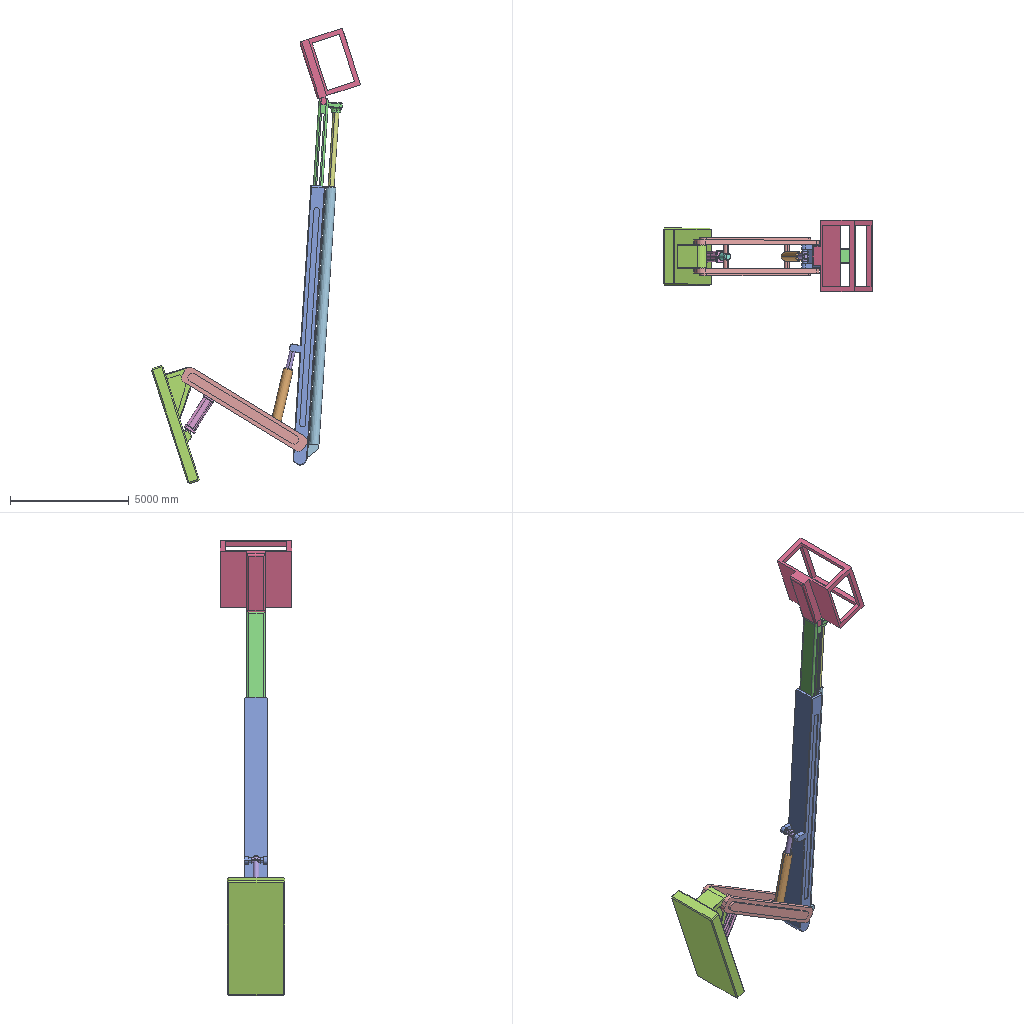Assembly | SolidWorks | 11 different items | 11 placed | box 8811 x 3000 x 19206 mm
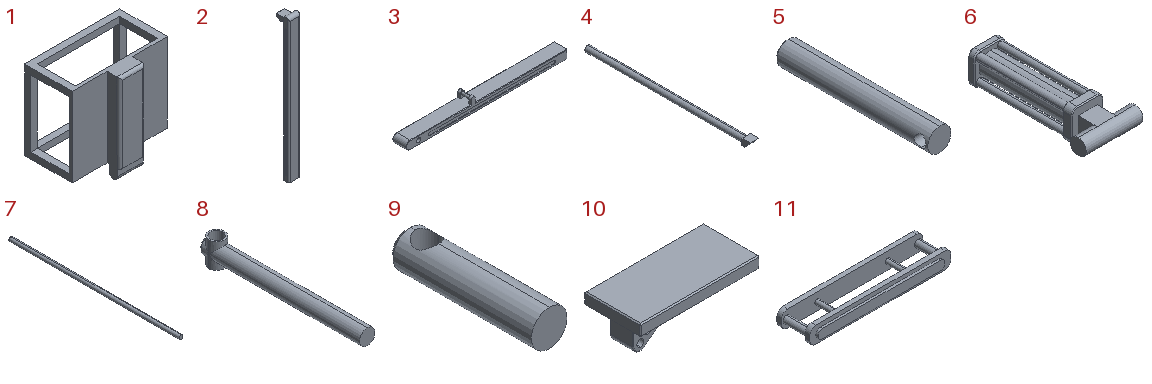Parts list (item | quantity | size | volume | features):
1 | x1 | 3000 x 1900 x 2845 mm | 2208765977 mm3 | features ICE 6, Extrusion 1, Fillet 1
2 | x1 | 800 x 1000 x 10000 mm | 2403832717 mm3 | features ICE 9, Fillet 2, Chamfer 1, Extrusion 1
3 | x1 | 11800 x 1000 x 1050 mm | 3596750717 mm3 | features ICE 4, Chamfer 2, MirrorPattern 2, Extrusion 1
4 | x1 | 600 x 11470 x 450 mm | 1002202960 mm3 | features ICE 2, Chamfer 1, Extrusion 1
5 | x1 | 410 x 2700 x 410 mm | 230530673 mm3 | features ICE 2, Chamfer 1, Extrusion 1
6 | x1 | 900 x 2075 x 500 mm | 199236991 mm3 | features ICE 5, Chamfer 2, CirPattern 1, Extrusion 1, Fillet 1
7 | x1 | 250 x 11200 x 250 mm | 549778714 mm3 | features Extrusion 1
8 | x1 | 250 x 2600 x 400 mm | 123717822 mm3 | features ICE 3, Chamfer 1, Extrusion 1
9 | x1 | 300 x 1200 x 300 mm | 75269036 mm3 | features ICE 2, Chamfer 1, Extrusion 1
10 | x1 | 5102 x 2411 x 1700 mm | 7041996598 mm3 | features ICE 6, Chamfer 3, MirrorPattern 2, Extrusion 1, Fillet 1
11 | x1 | 6002 x 1600 x 700 mm | 2271942121 mm3 | features ICE 3, Extrusion 1, Fillet 1, MirrorPattern 1
Mates (type | each side: item.copy, entity, surface, feature):
Concentric | 11.1 face cylinder Boss-Extrude4 | 3.1 face cylinder Boss-Extrude1
Coincident | 11.1 face plane Boss-Extrude5 | 3.1 face plane Boss-Extrude1
Concentric | 11.1 face cylinder Boss-Extrude4 | 10.1 face cylinder Boss-Extrude1
Coincident | 11.1 face plane Boss-Extrude5 | 10.1 face plane Boss-Extrude1
Concentric | 10.1 face cylinder Cut-Extrude1 | 6.1 face cylinder Boss-Extrude3
Coincident | 10.1 face plane Cut-Extrude1 | 6.1 face plane Boss-Extrude4
Concentric | 6.1 face cylinder Boss-Extrude1 | 9.1 face cylinder Boss-Extrude1
Concentric | 11.1 face cylinder Boss-Extrude4 | 9.1 face cylinder Cut-Extrude1
Concentric | 11.1 face cylinder Boss-Extrude4 | 5.1 face cylinder Cut-Extrude1
Concentric | 3.1 face cylinder Boss-Extrude3 | 8.1 face cylinder Cut-Extrude1
Concentric | 5.1 face cylinder Boss-Extrude1 | 8.1 face cylinder Boss-Extrude1
DistanceDim | 8.1 face plane Boss-Extrude2 | 3.1 face plane Boss-Extrude2
Coincident | 3.1 face plane Cut-Extrude1 | 2.1 face plane Boss-Extrude1 | 2 times
Concentric | 2.1 face cylinder Cut-Extrude5 | 1.1 face cylinder Boss-Extrude3
Coincident | 2.1 face plane Boss-Extrude1 | 1.1 face plane Boss-Extrude1
Parallel | 10.1 face plane Boss-Extrude2 | 1.1 face plane Boss-Extrude1
Concentric | 2.1 face cylinder Boss-Extrude4 | 7.1 face cylinder Boss-Extrude1
Coincident | 2.1 face plane Boss-Extrude3 | 7.1 face plane Boss-Extrude1
Concentric | 4.1 face cylinder Boss-Extrude1 | 7.1 face cylinder Boss-Extrude1
Parallel | 3.1 face plane Boss-Extrude1 | 4.1 face plane Boss-Extrude3
DistanceDim | 4.1 face plane Boss-Extrude1 | 3.1 face plane Boss-Extrude1